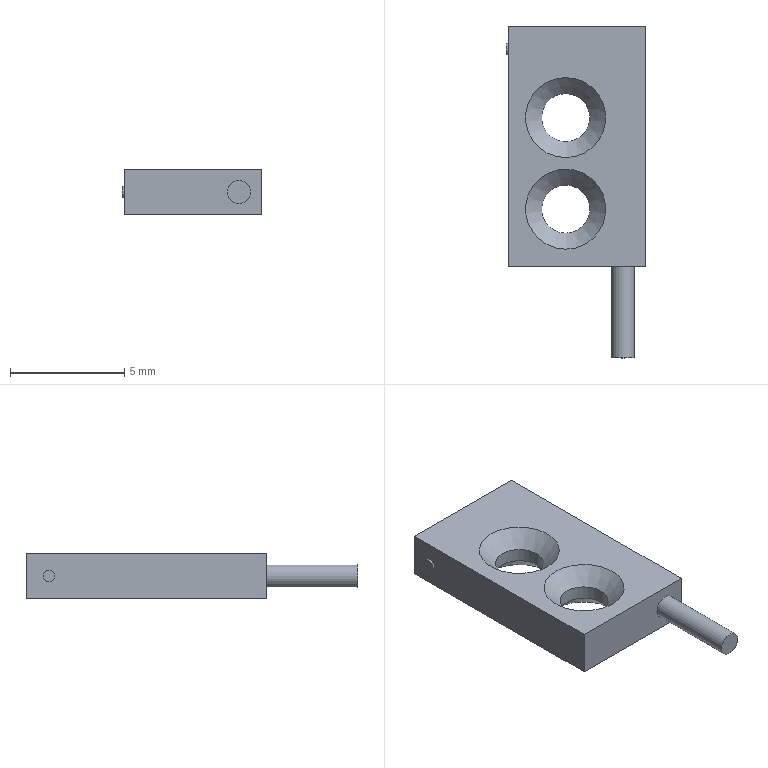Part | NX | features 倒角1 2 | 1 solid | 16 faces | box 6.1 x 14.5 x 2 mm | volume 107.405 mm3 | plane 8 | cone 4 | cylinder 4 | commonest cylinder face diameters 2.1 x2 0.5 x1 1 x1
STEP:
#1=CARTESIAN_POINT('',(56.5,91.25,-80.5));
#2=VERTEX_POINT('',#1);
#3=CARTESIAN_POINT('',(56.5,93.,-80.5));
#4=DIRECTION('',(0.,0.,-1.));
#5=DIRECTION('',(0.,-1.,0.));
#6=AXIS2_PLACEMENT_3D('',#3,#4,#5);
#7=CIRCLE('',#6,1.75);
#8=EDGE_CURVE('',#2,#2,#7,.T.);
#9=ORIENTED_EDGE('',*,*,#8,.F.);
#10=EDGE_LOOP('',(#9));
#11=FACE_BOUND('',#10,.T.);
#12=CARTESIAN_POINT('',(56.5,91.95,-81.2));
#13=VERTEX_POINT('',#12);
#14=CARTESIAN_POINT('',(56.5,93.,-81.2));
#15=DIRECTION('',(0.,0.,1.));
#16=DIRECTION('',(0.,-1.,0.));
#17=AXIS2_PLACEMENT_3D('',#14,#15,#16);
#18=CIRCLE('',#17,1.05);
#19=EDGE_CURVE('',#13,#13,#18,.T.);
#20=ORIENTED_EDGE('',*,*,#19,.F.);
#21=EDGE_LOOP('',(#20));
#22=FACE_BOUND('',#21,.T.);
#23=CARTESIAN_POINT('',(56.5,93.,-80.5));
#24=DIRECTION('',(0.,0.,1.));
#25=DIRECTION('',(0.,-1.,0.));
#26=AXIS2_PLACEMENT_3D('',#23,#24,#25);
#27=CONICAL_SURFACE('',#26,1.75,0.7854);
#28=ADVANCED_FACE('',(#11,#22),#27,.F.);
#29=CARTESIAN_POINT('',(56.5,95.25,-80.5));
#30=VERTEX_POINT('',#29);
#31=CARTESIAN_POINT('',(56.5,97.,-80.5));
#32=DIRECTION('',(0.,0.,-1.));
#33=DIRECTION('',(0.,-1.,0.));
#34=AXIS2_PLACEMENT_3D('',#31,#32,#33);
#35=CIRCLE('',#34,1.75);
#36=EDGE_CURVE('',#30,#30,#35,.T.);
#37=ORIENTED_EDGE('',*,*,#36,.F.);
#38=EDGE_LOOP('',(#37));
#39=FACE_BOUND('',#38,.T.);
#40=CARTESIAN_POINT('',(56.5,95.95,-81.2));
#41=VERTEX_POINT('',#40);
#42=CARTESIAN_POINT('',(56.5,97.,-81.2));
#43=DIRECTION('',(0.,0.,1.));
#44=DIRECTION('',(0.,-1.,0.));
#45=AXIS2_PLACEMENT_3D('',#42,#43,#44);
#46=CIRCLE('',#45,1.05);
#47=EDGE_CURVE('',#41,#41,#46,.T.);
#48=ORIENTED_EDGE('',*,*,#47,.F.);
#49=EDGE_LOOP('',(#48));
#50=FACE_BOUND('',#49,.T.);
#51=CARTESIAN_POINT('',(56.5,97.,-80.5));
#52=DIRECTION('',(0.,0.,1.));
#53=DIRECTION('',(0.,-1.,0.));
#54=AXIS2_PLACEMENT_3D('',#51,#52,#53);
#55=CONICAL_SURFACE('',#54,1.75,0.7854);
#56=ADVANCED_FACE('',(#39,#50),#55,.F.);
#57=CARTESIAN_POINT('',(54.,100.,-81.25));
#58=VERTEX_POINT('',#57);
#59=CARTESIAN_POINT('',(54.,100.,-81.5));
#60=DIRECTION('',(-1.,0.,0.));
#61=DIRECTION('',(0.,0.,1.));
#62=AXIS2_PLACEMENT_3D('',#59,#60,#61);
#63=CIRCLE('',#62,0.25);
#64=EDGE_CURVE('',#58,#58,#63,.T.);
#65=ORIENTED_EDGE('',*,*,#64,.T.);
#66=EDGE_LOOP('',(#65));
#67=FACE_BOUND('',#66,.T.);
#68=CARTESIAN_POINT('',(53.9,100.,-81.75));
#69=VERTEX_POINT('',#68);
#70=CARTESIAN_POINT('',(53.9,100.,-81.5));
#71=DIRECTION('',(-1.,0.,0.));
#72=DIRECTION('',(0.,0.,-1.));
#73=AXIS2_PLACEMENT_3D('',#70,#71,#72);
#74=CIRCLE('',#73,0.25);
#75=EDGE_CURVE('',#69,#69,#74,.T.);
#76=ORIENTED_EDGE('',*,*,#75,.F.);
#77=EDGE_LOOP('',(#76));
#78=FACE_BOUND('',#77,.T.);
#79=CARTESIAN_POINT('',(53.9,100.,-81.5));
#80=DIRECTION('',(1.,0.,0.));
#81=DIRECTION('',(0.,0.,-1.));
#82=AXIS2_PLACEMENT_3D('',#79,#80,#81);
#83=CYLINDRICAL_SURFACE('',#82,0.25);
#84=ADVANCED_FACE('',(#67,#78),#83,.T.);
#85=CARTESIAN_POINT('',(59.5,90.5,-81.5));
#86=VERTEX_POINT('',#85);
#87=CARTESIAN_POINT('',(59.,90.5,-81.5));
#88=DIRECTION('',(0.,-1.,0.));
#89=DIRECTION('',(1.,0.,0.));
#90=AXIS2_PLACEMENT_3D('',#87,#88,#89);
#91=CIRCLE('',#90,0.5);
#92=EDGE_CURVE('',#86,#86,#91,.T.);
#93=ORIENTED_EDGE('',*,*,#92,.T.);
#94=EDGE_LOOP('',(#93));
#95=FACE_BOUND('',#94,.T.);
#96=CARTESIAN_POINT('',(58.5,86.5,-81.5));
#97=VERTEX_POINT('',#96);
#98=CARTESIAN_POINT('',(59.,86.5,-81.5));
#99=DIRECTION('',(0.,-1.,0.));
#100=DIRECTION('',(-1.,0.,0.));
#101=AXIS2_PLACEMENT_3D('',#98,#99,#100);
#102=CIRCLE('',#101,0.5);
#103=EDGE_CURVE('',#97,#97,#102,.T.);
#104=ORIENTED_EDGE('',*,*,#103,.F.);
#105=EDGE_LOOP('',(#104));
#106=FACE_BOUND('',#105,.T.);
#107=CARTESIAN_POINT('',(59.,86.5,-81.5));
#108=DIRECTION('',(0.,1.,0.));
#109=DIRECTION('',(-1.,0.,0.));
#110=AXIS2_PLACEMENT_3D('',#107,#108,#109);
#111=CYLINDRICAL_SURFACE('',#110,0.5);
#112=ADVANCED_FACE('',(#95,#106),#111,.T.);
#113=CARTESIAN_POINT('',(56.5,91.25,-82.5));
#114=VERTEX_POINT('',#113);
#115=CARTESIAN_POINT('',(56.5,93.,-82.5));
#116=DIRECTION('',(0.,0.,-1.));
#117=DIRECTION('',(0.,-1.,0.));
#118=AXIS2_PLACEMENT_3D('',#115,#116,#117);
#119=CIRCLE('',#118,1.75);
#120=EDGE_CURVE('',#114,#114,#119,.T.);
#121=ORIENTED_EDGE('',*,*,#120,.T.);
#122=EDGE_LOOP('',(#121));
#123=FACE_BOUND('',#122,.T.);
#124=CARTESIAN_POINT('',(56.5,91.95,-81.8));
#125=VERTEX_POINT('',#124);
#126=CARTESIAN_POINT('',(56.5,93.,-81.8));
#127=DIRECTION('',(0.,0.,-1.));
#128=DIRECTION('',(0.,-1.,0.));
#129=AXIS2_PLACEMENT_3D('',#126,#127,#128);
#130=CIRCLE('',#129,1.05);
#131=EDGE_CURVE('',#125,#125,#130,.T.);
#132=ORIENTED_EDGE('',*,*,#131,.F.);
#133=EDGE_LOOP('',(#132));
#134=FACE_BOUND('',#133,.T.);
#135=CARTESIAN_POINT('',(56.5,93.,-82.5));
#136=DIRECTION('',(0.,0.,-1.));
#137=DIRECTION('',(0.,1.,0.));
#138=AXIS2_PLACEMENT_3D('',#135,#136,#137);
#139=CONICAL_SURFACE('',#138,1.75,0.7854);
#140=ADVANCED_FACE('',(#123,#134),#139,.F.);
#141=ORIENTED_EDGE('',*,*,#131,.T.);
#142=EDGE_LOOP('',(#141));
#143=FACE_BOUND('',#142,.T.);
#144=ORIENTED_EDGE('',*,*,#19,.T.);
#145=EDGE_LOOP('',(#144));
#146=FACE_BOUND('',#145,.T.);
#147=CARTESIAN_POINT('',(56.5,93.,-82.5));
#148=DIRECTION('',(0.,0.,-1.));
#149=DIRECTION('',(0.,1.,0.));
#150=AXIS2_PLACEMENT_3D('',#147,#148,#149);
#151=CYLINDRICAL_SURFACE('',#150,1.05);
#152=ADVANCED_FACE('',(#143,#146),#151,.F.);
#153=CARTESIAN_POINT('',(56.5,95.25,-82.5));
#154=VERTEX_POINT('',#153);
#155=CARTESIAN_POINT('',(56.5,97.,-82.5));
#156=DIRECTION('',(0.,0.,-1.));
#157=DIRECTION('',(0.,-1.,0.));
#158=AXIS2_PLACEMENT_3D('',#155,#156,#157);
#159=CIRCLE('',#158,1.75);
#160=EDGE_CURVE('',#154,#154,#159,.T.);
#161=ORIENTED_EDGE('',*,*,#160,.T.);
#162=EDGE_LOOP('',(#161));
#163=FACE_BOUND('',#162,.T.);
#164=CARTESIAN_POINT('',(56.5,95.95,-81.8));
#165=VERTEX_POINT('',#164);
#166=CARTESIAN_POINT('',(56.5,97.,-81.8));
#167=DIRECTION('',(0.,0.,-1.));
#168=DIRECTION('',(0.,-1.,0.));
#169=AXIS2_PLACEMENT_3D('',#166,#167,#168);
#170=CIRCLE('',#169,1.05);
#171=EDGE_CURVE('',#165,#165,#170,.T.);
#172=ORIENTED_EDGE('',*,*,#171,.F.);
#173=EDGE_LOOP('',(#172));
#174=FACE_BOUND('',#173,.T.);
#175=CARTESIAN_POINT('',(56.5,97.,-82.5));
#176=DIRECTION('',(0.,0.,-1.));
#177=DIRECTION('',(0.,1.,0.));
#178=AXIS2_PLACEMENT_3D('',#175,#176,#177);
#179=CONICAL_SURFACE('',#178,1.75,0.7854);
#180=ADVANCED_FACE('',(#163,#174),#179,.F.);
#181=ORIENTED_EDGE('',*,*,#171,.T.);
#182=EDGE_LOOP('',(#181));
#183=FACE_BOUND('',#182,.T.);
#184=ORIENTED_EDGE('',*,*,#47,.T.);
#185=EDGE_LOOP('',(#184));
#186=FACE_BOUND('',#185,.T.);
#187=CARTESIAN_POINT('',(56.5,97.,-82.5));
#188=DIRECTION('',(0.,0.,-1.));
#189=DIRECTION('',(0.,1.,0.));
#190=AXIS2_PLACEMENT_3D('',#187,#188,#189);
#191=CYLINDRICAL_SURFACE('',#190,1.05);
#192=ADVANCED_FACE('',(#183,#186),#191,.F.);
#193=ORIENTED_EDGE('',*,*,#92,.F.);
#194=EDGE_LOOP('',(#193));
#195=FACE_BOUND('',#194,.T.);
#196=CARTESIAN_POINT('',(60.,90.5,-80.5));
#197=VERTEX_POINT('',#196);
#198=CARTESIAN_POINT('',(54.,90.5,-80.5));
#199=VERTEX_POINT('',#198);
#200=CARTESIAN_POINT('',(54.,90.5,-80.5));
#201=DIRECTION('',(-1.,0.,0.));
#202=VECTOR('',#201,1000.);
#203=LINE('',#200,#202);
#204=EDGE_CURVE('',#197,#199,#203,.T.);
#205=ORIENTED_EDGE('',*,*,#204,.T.);
#206=CARTESIAN_POINT('',(54.,90.5,-82.5));
#207=VERTEX_POINT('',#206);
#208=CARTESIAN_POINT('',(54.,90.5,-82.5));
#209=DIRECTION('',(0.,0.,1.));
#210=VECTOR('',#209,1000.);
#211=LINE('',#208,#210);
#212=EDGE_CURVE('',#207,#199,#211,.T.);
#213=ORIENTED_EDGE('',*,*,#212,.F.);
#214=CARTESIAN_POINT('',(60.,90.5,-82.5));
#215=VERTEX_POINT('',#214);
#216=CARTESIAN_POINT('',(54.,90.5,-82.5));
#217=DIRECTION('',(-1.,0.,0.));
#218=VECTOR('',#217,1000.);
#219=LINE('',#216,#218);
#220=EDGE_CURVE('',#215,#207,#219,.T.);
#221=ORIENTED_EDGE('',*,*,#220,.F.);
#222=CARTESIAN_POINT('',(60.,90.5,-82.5));
#223=DIRECTION('',(0.,0.,1.));
#224=VECTOR('',#223,1000.);
#225=LINE('',#222,#224);
#226=EDGE_CURVE('',#215,#197,#225,.T.);
#227=ORIENTED_EDGE('',*,*,#226,.T.);
#228=EDGE_LOOP('',(#205,#213,#221,#227));
#229=FACE_BOUND('',#228,.T.);
#230=CARTESIAN_POINT('',(54.,90.5,-82.5));
#231=DIRECTION('',(0.,1.,0.));
#232=DIRECTION('',(-1.,0.,0.));
#233=AXIS2_PLACEMENT_3D('',#230,#231,#232);
#234=PLANE('',#233);
#235=ADVANCED_FACE('',(#195,#229),#234,.F.);
#236=ORIENTED_EDGE('',*,*,#64,.F.);
#237=EDGE_LOOP('',(#236));
#238=FACE_BOUND('',#237,.T.);
#239=CARTESIAN_POINT('',(54.,101.,-80.5));
#240=VERTEX_POINT('',#239);
#241=CARTESIAN_POINT('',(54.,101.,-80.5));
#242=DIRECTION('',(0.,1.,0.));
#243=VECTOR('',#242,1000.);
#244=LINE('',#241,#243);
#245=EDGE_CURVE('',#199,#240,#244,.T.);
#246=ORIENTED_EDGE('',*,*,#245,.T.);
#247=CARTESIAN_POINT('',(54.,101.,-82.5));
#248=VERTEX_POINT('',#247);
#249=CARTESIAN_POINT('',(54.,101.,-82.5));
#250=DIRECTION('',(0.,0.,1.));
#251=VECTOR('',#250,1000.);
#252=LINE('',#249,#251);
#253=EDGE_CURVE('',#248,#240,#252,.T.);
#254=ORIENTED_EDGE('',*,*,#253,.F.);
#255=CARTESIAN_POINT('',(54.,101.,-82.5));
#256=DIRECTION('',(0.,1.,0.));
#257=VECTOR('',#256,1000.);
#258=LINE('',#255,#257);
#259=EDGE_CURVE('',#207,#248,#258,.T.);
#260=ORIENTED_EDGE('',*,*,#259,.F.);
#261=ORIENTED_EDGE('',*,*,#212,.T.);
#262=EDGE_LOOP('',(#246,#254,#260,#261));
#263=FACE_BOUND('',#262,.T.);
#264=CARTESIAN_POINT('',(54.,101.,-82.5));
#265=DIRECTION('',(1.,0.,0.));
#266=DIRECTION('',(0.,0.,-1.));
#267=AXIS2_PLACEMENT_3D('',#264,#265,#266);
#268=PLANE('',#267);
#269=ADVANCED_FACE('',(#238,#263),#268,.F.);
#270=CARTESIAN_POINT('',(60.,101.,-80.5));
#271=VERTEX_POINT('',#270);
#272=CARTESIAN_POINT('',(54.,101.,-80.5));
#273=DIRECTION('',(1.,0.,0.));
#274=VECTOR('',#273,1000.);
#275=LINE('',#272,#274);
#276=EDGE_CURVE('',#240,#271,#275,.T.);
#277=ORIENTED_EDGE('',*,*,#276,.T.);
#278=CARTESIAN_POINT('',(60.,101.,-82.5));
#279=VERTEX_POINT('',#278);
#280=CARTESIAN_POINT('',(60.,101.,-82.5));
#281=DIRECTION('',(0.,0.,1.));
#282=VECTOR('',#281,1000.);
#283=LINE('',#280,#282);
#284=EDGE_CURVE('',#279,#271,#283,.T.);
#285=ORIENTED_EDGE('',*,*,#284,.F.);
#286=CARTESIAN_POINT('',(54.,101.,-82.5));
#287=DIRECTION('',(1.,0.,0.));
#288=VECTOR('',#287,1000.);
#289=LINE('',#286,#288);
#290=EDGE_CURVE('',#248,#279,#289,.T.);
#291=ORIENTED_EDGE('',*,*,#290,.F.);
#292=ORIENTED_EDGE('',*,*,#253,.T.);
#293=EDGE_LOOP('',(#277,#285,#291,#292));
#294=FACE_BOUND('',#293,.T.);
#295=CARTESIAN_POINT('',(54.,101.,-82.5));
#296=DIRECTION('',(0.,-1.,0.));
#297=DIRECTION('',(0.,0.,-1.));
#298=AXIS2_PLACEMENT_3D('',#295,#296,#297);
#299=PLANE('',#298);
#300=ADVANCED_FACE('',(#294),#299,.F.);
#301=CARTESIAN_POINT('',(60.,101.,-80.5));
#302=DIRECTION('',(0.,-1.,0.));
#303=VECTOR('',#302,1000.);
#304=LINE('',#301,#303);
#305=EDGE_CURVE('',#271,#197,#304,.T.);
#306=ORIENTED_EDGE('',*,*,#305,.T.);
#307=ORIENTED_EDGE('',*,*,#226,.F.);
#308=CARTESIAN_POINT('',(60.,101.,-82.5));
#309=DIRECTION('',(0.,-1.,0.));
#310=VECTOR('',#309,1000.);
#311=LINE('',#308,#310);
#312=EDGE_CURVE('',#279,#215,#311,.T.);
#313=ORIENTED_EDGE('',*,*,#312,.F.);
#314=ORIENTED_EDGE('',*,*,#284,.T.);
#315=EDGE_LOOP('',(#306,#307,#313,#314));
#316=FACE_BOUND('',#315,.T.);
#317=CARTESIAN_POINT('',(60.,101.,-82.5));
#318=DIRECTION('',(-1.,0.,0.));
#319=DIRECTION('',(0.,0.,1.));
#320=AXIS2_PLACEMENT_3D('',#317,#318,#319);
#321=PLANE('',#320);
#322=ADVANCED_FACE('',(#316),#321,.F.);
#323=ORIENTED_EDGE('',*,*,#120,.F.);
#324=EDGE_LOOP('',(#323));
#325=FACE_BOUND('',#324,.T.);
#326=ORIENTED_EDGE('',*,*,#160,.F.);
#327=EDGE_LOOP('',(#326));
#328=FACE_BOUND('',#327,.T.);
#329=ORIENTED_EDGE('',*,*,#220,.T.);
#330=ORIENTED_EDGE('',*,*,#259,.T.);
#331=ORIENTED_EDGE('',*,*,#290,.T.);
#332=ORIENTED_EDGE('',*,*,#312,.T.);
#333=EDGE_LOOP('',(#329,#330,#331,#332));
#334=FACE_BOUND('',#333,.T.);
#335=CARTESIAN_POINT('',(57.,95.75,-82.5));
#336=DIRECTION('',(0.,0.,-1.));
#337=DIRECTION('',(0.,1.,0.));
#338=AXIS2_PLACEMENT_3D('',#335,#336,#337);
#339=PLANE('',#338);
#340=ADVANCED_FACE('',(#325,#328,#334),#339,.T.);
#341=ORIENTED_EDGE('',*,*,#36,.T.);
#342=EDGE_LOOP('',(#341));
#343=FACE_BOUND('',#342,.T.);
#344=ORIENTED_EDGE('',*,*,#8,.T.);
#345=EDGE_LOOP('',(#344));
#346=FACE_BOUND('',#345,.T.);
#347=ORIENTED_EDGE('',*,*,#204,.F.);
#348=ORIENTED_EDGE('',*,*,#305,.F.);
#349=ORIENTED_EDGE('',*,*,#276,.F.);
#350=ORIENTED_EDGE('',*,*,#245,.F.);
#351=EDGE_LOOP('',(#347,#348,#349,#350));
#352=FACE_BOUND('',#351,.T.);
#353=CARTESIAN_POINT('',(57.,95.75,-80.5));
#354=DIRECTION('',(0.,0.,-1.));
#355=DIRECTION('',(0.,1.,0.));
#356=AXIS2_PLACEMENT_3D('',#353,#354,#355);
#357=PLANE('',#356);
#358=ADVANCED_FACE('',(#343,#346,#352),#357,.F.);
#359=ORIENTED_EDGE('',*,*,#103,.T.);
#360=EDGE_LOOP('',(#359));
#361=FACE_BOUND('',#360,.T.);
#362=CARTESIAN_POINT('',(59.,86.5,-81.5));
#363=DIRECTION('',(0.,-1.,0.));
#364=DIRECTION('',(1.,0.,0.));
#365=AXIS2_PLACEMENT_3D('',#362,#363,#364);
#366=PLANE('',#365);
#367=ADVANCED_FACE('',(#361),#366,.T.);
#368=ORIENTED_EDGE('',*,*,#75,.T.);
#369=EDGE_LOOP('',(#368));
#370=FACE_BOUND('',#369,.T.);
#371=CARTESIAN_POINT('',(53.9,100.,-81.5));
#372=DIRECTION('',(-1.,0.,0.));
#373=DIRECTION('',(0.,0.,1.));
#374=AXIS2_PLACEMENT_3D('',#371,#372,#373);
#375=PLANE('',#374);
#376=ADVANCED_FACE('',(#370),#375,.T.);
#377=CLOSED_SHELL('',(#28,#56,#84,#112,#140,#152,#180,#192,#235,#269,#300,#322,#340,#358,#367,#376));
#378=MANIFOLD_SOLID_BREP('',#377);
#379=(LENGTH_UNIT()NAMED_UNIT(*)SI_UNIT(.MILLI.,.METRE.));
#380=UNCERTAINTY_MEASURE_WITH_UNIT(LENGTH_MEASURE(0.00001),#379,'','');
#381=(NAMED_UNIT(*)PLANE_ANGLE_UNIT()SI_UNIT($,.RADIAN.));
#382=(NAMED_UNIT(*)SI_UNIT($,.STERADIAN.)SOLID_ANGLE_UNIT());
#383=(GEOMETRIC_REPRESENTATION_CONTEXT(3)GLOBAL_UNCERTAINTY_ASSIGNED_CONTEXT((#380))GLOBAL_UNIT_ASSIGNED_CONTEXT((#379,#381,#382))REPRESENTATION_CONTEXT('',''));
#384=ADVANCED_BREP_SHAPE_REPRESENTATION('',(#378),#383);